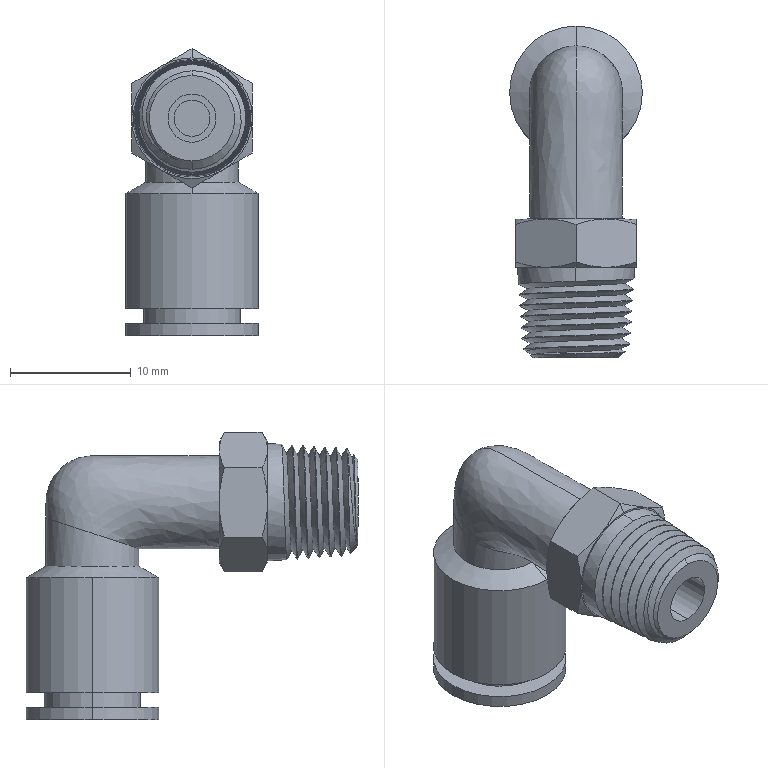Part | 1 solid | 75 faces | box 11 x 27.5 x 23.774 mm | volume 2298 mm3 | cone 31 | plane 20 | cylinder 18 | spline 6 | commonest cylinder face diameters 4 x4 11 x4 3 x2 8 x2 8.2 x2 10.2 x2